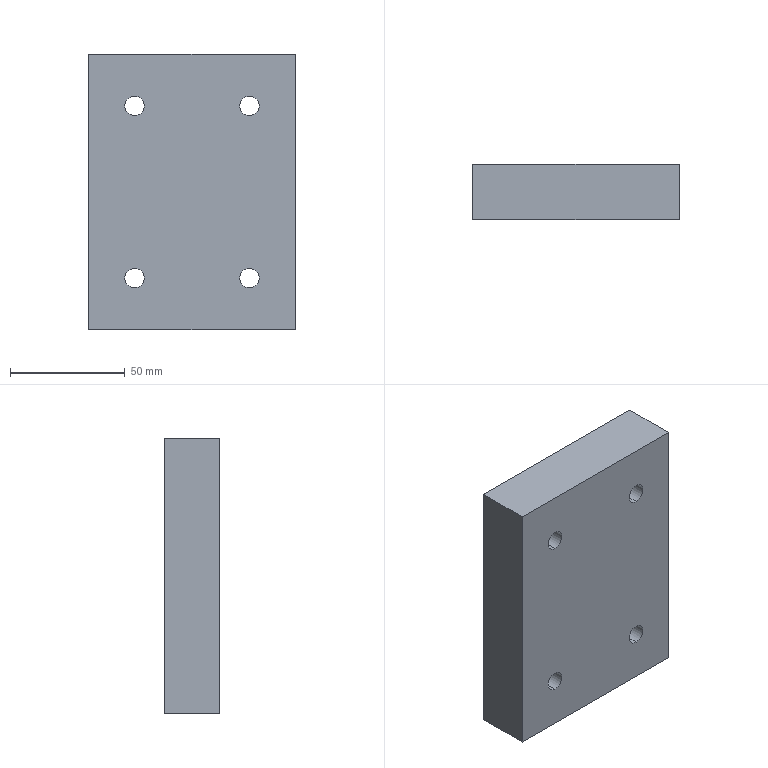Part | SolidWorks | features Extrusion 1, HoleWzd 1 | 1 solid | 14 faces | box 90 x 24 x 120 mm | volume 253752 mm3 | cylinder 8 | plane 6 | commonest cylinder face diameters 8.5 x8
STEP:
#1=CARTESIAN_POINT('',(-25.,0.,33.25));
#2=VERTEX_POINT('',#1);
#3=CARTESIAN_POINT('',(-25.,0.,41.75));
#4=VERTEX_POINT('',#3);
#5=CARTESIAN_POINT('',(-25.,0.,37.5));
#6=DIRECTION('',(0.,1.,0.));
#7=DIRECTION('',(0.,0.,1.));
#8=AXIS2_PLACEMENT_3D('',#5,#6,#7);
#9=CIRCLE('',#8,4.25);
#10=EDGE_CURVE('',#2,#4,#9,.T.);
#11=ORIENTED_EDGE('',*,*,#10,.F.);
#12=CARTESIAN_POINT('',(-25.,24.,33.25));
#13=VERTEX_POINT('',#12);
#14=CARTESIAN_POINT('',(-25.,24.,33.25));
#15=DIRECTION('',(0.,1.,0.));
#16=VECTOR('',#15,1000.);
#17=LINE('',#14,#16);
#18=EDGE_CURVE('',#2,#13,#17,.T.);
#19=ORIENTED_EDGE('',*,*,#18,.T.);
#20=CARTESIAN_POINT('',(-25.,24.,41.75));
#21=VERTEX_POINT('',#20);
#22=CARTESIAN_POINT('',(-25.,24.,37.5));
#23=DIRECTION('',(0.,1.,0.));
#24=DIRECTION('',(0.,0.,1.));
#25=AXIS2_PLACEMENT_3D('',#22,#23,#24);
#26=CIRCLE('',#25,4.25);
#27=EDGE_CURVE('',#13,#21,#26,.T.);
#28=ORIENTED_EDGE('',*,*,#27,.T.);
#29=CARTESIAN_POINT('',(-25.,24.,41.75));
#30=DIRECTION('',(0.,1.,0.));
#31=VECTOR('',#30,1000.);
#32=LINE('',#29,#31);
#33=EDGE_CURVE('',#4,#21,#32,.T.);
#34=ORIENTED_EDGE('',*,*,#33,.F.);
#35=EDGE_LOOP('',(#11,#19,#28,#34));
#36=FACE_OUTER_BOUND('',#35,.T.);
#37=CARTESIAN_POINT('',(-25.,24.,37.5));
#38=DIRECTION('',(0.,1.,0.));
#39=DIRECTION('',(0.,0.,1.));
#40=AXIS2_PLACEMENT_3D('',#37,#38,#39);
#41=CYLINDRICAL_SURFACE('',#40,4.25);
#42=ADVANCED_FACE('',(#36),#41,.F.);
#43=CARTESIAN_POINT('',(-25.,0.,-41.75));
#44=VERTEX_POINT('',#43);
#45=CARTESIAN_POINT('',(-25.,0.,-33.25));
#46=VERTEX_POINT('',#45);
#47=CARTESIAN_POINT('',(-25.,0.,-37.5));
#48=DIRECTION('',(0.,1.,0.));
#49=DIRECTION('',(0.,0.,1.));
#50=AXIS2_PLACEMENT_3D('',#47,#48,#49);
#51=CIRCLE('',#50,4.25);
#52=EDGE_CURVE('',#44,#46,#51,.T.);
#53=ORIENTED_EDGE('',*,*,#52,.F.);
#54=CARTESIAN_POINT('',(-25.,24.,-41.75));
#55=VERTEX_POINT('',#54);
#56=CARTESIAN_POINT('',(-25.,24.,-41.75));
#57=DIRECTION('',(0.,1.,0.));
#58=VECTOR('',#57,1000.);
#59=LINE('',#56,#58);
#60=EDGE_CURVE('',#44,#55,#59,.T.);
#61=ORIENTED_EDGE('',*,*,#60,.T.);
#62=CARTESIAN_POINT('',(-25.,24.,-33.25));
#63=VERTEX_POINT('',#62);
#64=CARTESIAN_POINT('',(-25.,24.,-37.5));
#65=DIRECTION('',(0.,1.,0.));
#66=DIRECTION('',(0.,0.,1.));
#67=AXIS2_PLACEMENT_3D('',#64,#65,#66);
#68=CIRCLE('',#67,4.25);
#69=EDGE_CURVE('',#55,#63,#68,.T.);
#70=ORIENTED_EDGE('',*,*,#69,.T.);
#71=CARTESIAN_POINT('',(-25.,24.,-33.25));
#72=DIRECTION('',(0.,1.,0.));
#73=VECTOR('',#72,1000.);
#74=LINE('',#71,#73);
#75=EDGE_CURVE('',#46,#63,#74,.T.);
#76=ORIENTED_EDGE('',*,*,#75,.F.);
#77=EDGE_LOOP('',(#53,#61,#70,#76));
#78=FACE_OUTER_BOUND('',#77,.T.);
#79=CARTESIAN_POINT('',(-25.,24.,-37.5));
#80=DIRECTION('',(0.,1.,0.));
#81=DIRECTION('',(0.,0.,1.));
#82=AXIS2_PLACEMENT_3D('',#79,#80,#81);
#83=CYLINDRICAL_SURFACE('',#82,4.25);
#84=ADVANCED_FACE('',(#78),#83,.F.);
#85=CARTESIAN_POINT('',(25.,0.,-41.75));
#86=VERTEX_POINT('',#85);
#87=CARTESIAN_POINT('',(25.,0.,-33.25));
#88=VERTEX_POINT('',#87);
#89=CARTESIAN_POINT('',(25.,0.,-37.5));
#90=DIRECTION('',(0.,1.,0.));
#91=DIRECTION('',(0.,0.,1.));
#92=AXIS2_PLACEMENT_3D('',#89,#90,#91);
#93=CIRCLE('',#92,4.25);
#94=EDGE_CURVE('',#86,#88,#93,.T.);
#95=ORIENTED_EDGE('',*,*,#94,.F.);
#96=CARTESIAN_POINT('',(25.,24.,-41.75));
#97=VERTEX_POINT('',#96);
#98=CARTESIAN_POINT('',(25.,24.,-41.75));
#99=DIRECTION('',(0.,1.,0.));
#100=VECTOR('',#99,1000.);
#101=LINE('',#98,#100);
#102=EDGE_CURVE('',#86,#97,#101,.T.);
#103=ORIENTED_EDGE('',*,*,#102,.T.);
#104=CARTESIAN_POINT('',(25.,24.,-33.25));
#105=VERTEX_POINT('',#104);
#106=CARTESIAN_POINT('',(25.,24.,-37.5));
#107=DIRECTION('',(0.,1.,0.));
#108=DIRECTION('',(0.,0.,1.));
#109=AXIS2_PLACEMENT_3D('',#106,#107,#108);
#110=CIRCLE('',#109,4.25);
#111=EDGE_CURVE('',#97,#105,#110,.T.);
#112=ORIENTED_EDGE('',*,*,#111,.T.);
#113=CARTESIAN_POINT('',(25.,24.,-33.25));
#114=DIRECTION('',(0.,1.,0.));
#115=VECTOR('',#114,1000.);
#116=LINE('',#113,#115);
#117=EDGE_CURVE('',#88,#105,#116,.T.);
#118=ORIENTED_EDGE('',*,*,#117,.F.);
#119=EDGE_LOOP('',(#95,#103,#112,#118));
#120=FACE_OUTER_BOUND('',#119,.T.);
#121=CARTESIAN_POINT('',(25.,24.,-37.5));
#122=DIRECTION('',(0.,1.,0.));
#123=DIRECTION('',(0.,0.,1.));
#124=AXIS2_PLACEMENT_3D('',#121,#122,#123);
#125=CYLINDRICAL_SURFACE('',#124,4.25);
#126=ADVANCED_FACE('',(#120),#125,.F.);
#127=CARTESIAN_POINT('',(25.,0.,33.25));
#128=VERTEX_POINT('',#127);
#129=CARTESIAN_POINT('',(25.,0.,41.75));
#130=VERTEX_POINT('',#129);
#131=CARTESIAN_POINT('',(25.,0.,37.5));
#132=DIRECTION('',(0.,1.,0.));
#133=DIRECTION('',(0.,0.,1.));
#134=AXIS2_PLACEMENT_3D('',#131,#132,#133);
#135=CIRCLE('',#134,4.25);
#136=EDGE_CURVE('',#128,#130,#135,.T.);
#137=ORIENTED_EDGE('',*,*,#136,.F.);
#138=CARTESIAN_POINT('',(25.,24.,33.25));
#139=VERTEX_POINT('',#138);
#140=CARTESIAN_POINT('',(25.,24.,33.25));
#141=DIRECTION('',(0.,1.,0.));
#142=VECTOR('',#141,1000.);
#143=LINE('',#140,#142);
#144=EDGE_CURVE('',#128,#139,#143,.T.);
#145=ORIENTED_EDGE('',*,*,#144,.T.);
#146=CARTESIAN_POINT('',(25.,24.,41.75));
#147=VERTEX_POINT('',#146);
#148=CARTESIAN_POINT('',(25.,24.,37.5));
#149=DIRECTION('',(0.,1.,0.));
#150=DIRECTION('',(0.,0.,1.));
#151=AXIS2_PLACEMENT_3D('',#148,#149,#150);
#152=CIRCLE('',#151,4.25);
#153=EDGE_CURVE('',#139,#147,#152,.T.);
#154=ORIENTED_EDGE('',*,*,#153,.T.);
#155=CARTESIAN_POINT('',(25.,24.,41.75));
#156=DIRECTION('',(0.,1.,0.));
#157=VECTOR('',#156,1000.);
#158=LINE('',#155,#157);
#159=EDGE_CURVE('',#130,#147,#158,.T.);
#160=ORIENTED_EDGE('',*,*,#159,.F.);
#161=EDGE_LOOP('',(#137,#145,#154,#160));
#162=FACE_OUTER_BOUND('',#161,.T.);
#163=CARTESIAN_POINT('',(25.,24.,37.5));
#164=DIRECTION('',(0.,1.,0.));
#165=DIRECTION('',(0.,0.,1.));
#166=AXIS2_PLACEMENT_3D('',#163,#164,#165);
#167=CYLINDRICAL_SURFACE('',#166,4.25);
#168=ADVANCED_FACE('',(#162),#167,.F.);
#169=CARTESIAN_POINT('',(45.,0.,60.));
#170=VERTEX_POINT('',#169);
#171=CARTESIAN_POINT('',(45.,0.,-60.));
#172=VERTEX_POINT('',#171);
#173=CARTESIAN_POINT('',(45.,0.,60.));
#174=DIRECTION('',(0.,0.,-1.));
#175=VECTOR('',#174,1000.);
#176=LINE('',#173,#175);
#177=EDGE_CURVE('',#170,#172,#176,.T.);
#178=ORIENTED_EDGE('',*,*,#177,.T.);
#179=CARTESIAN_POINT('',(45.,24.,-60.));
#180=VERTEX_POINT('',#179);
#181=CARTESIAN_POINT('',(45.,24.,-60.));
#182=DIRECTION('',(0.,-1.,0.));
#183=VECTOR('',#182,1000.);
#184=LINE('',#181,#183);
#185=EDGE_CURVE('',#180,#172,#184,.T.);
#186=ORIENTED_EDGE('',*,*,#185,.F.);
#187=CARTESIAN_POINT('',(45.,24.,60.));
#188=VERTEX_POINT('',#187);
#189=CARTESIAN_POINT('',(45.,24.,60.));
#190=DIRECTION('',(0.,0.,-1.));
#191=VECTOR('',#190,1000.);
#192=LINE('',#189,#191);
#193=EDGE_CURVE('',#188,#180,#192,.T.);
#194=ORIENTED_EDGE('',*,*,#193,.F.);
#195=CARTESIAN_POINT('',(45.,24.,60.));
#196=DIRECTION('',(0.,-1.,0.));
#197=VECTOR('',#196,1000.);
#198=LINE('',#195,#197);
#199=EDGE_CURVE('',#188,#170,#198,.T.);
#200=ORIENTED_EDGE('',*,*,#199,.T.);
#201=EDGE_LOOP('',(#178,#186,#194,#200));
#202=FACE_OUTER_BOUND('',#201,.T.);
#203=CARTESIAN_POINT('',(45.,24.,60.));
#204=DIRECTION('',(-1.,0.,0.));
#205=DIRECTION('',(0.,0.,1.));
#206=AXIS2_PLACEMENT_3D('',#203,#204,#205);
#207=PLANE('',#206);
#208=ADVANCED_FACE('',(#202),#207,.F.);
#209=CARTESIAN_POINT('',(-45.,0.,-60.));
#210=VERTEX_POINT('',#209);
#211=CARTESIAN_POINT('',(-45.,0.,-60.));
#212=DIRECTION('',(-1.,0.,0.));
#213=VECTOR('',#212,1000.);
#214=LINE('',#211,#213);
#215=EDGE_CURVE('',#172,#210,#214,.T.);
#216=ORIENTED_EDGE('',*,*,#215,.T.);
#217=CARTESIAN_POINT('',(-45.,24.,-60.));
#218=VERTEX_POINT('',#217);
#219=CARTESIAN_POINT('',(-45.,24.,-60.));
#220=DIRECTION('',(0.,-1.,0.));
#221=VECTOR('',#220,1000.);
#222=LINE('',#219,#221);
#223=EDGE_CURVE('',#218,#210,#222,.T.);
#224=ORIENTED_EDGE('',*,*,#223,.F.);
#225=CARTESIAN_POINT('',(-45.,24.,-60.));
#226=DIRECTION('',(-1.,0.,0.));
#227=VECTOR('',#226,1000.);
#228=LINE('',#225,#227);
#229=EDGE_CURVE('',#180,#218,#228,.T.);
#230=ORIENTED_EDGE('',*,*,#229,.F.);
#231=ORIENTED_EDGE('',*,*,#185,.T.);
#232=EDGE_LOOP('',(#216,#224,#230,#231));
#233=FACE_OUTER_BOUND('',#232,.T.);
#234=CARTESIAN_POINT('',(-45.,24.,-60.));
#235=DIRECTION('',(0.,0.,1.));
#236=DIRECTION('',(1.,0.,0.));
#237=AXIS2_PLACEMENT_3D('',#234,#235,#236);
#238=PLANE('',#237);
#239=ADVANCED_FACE('',(#233),#238,.F.);
#240=CARTESIAN_POINT('',(-45.,0.,60.));
#241=VERTEX_POINT('',#240);
#242=CARTESIAN_POINT('',(-45.,0.,60.));
#243=DIRECTION('',(0.,0.,1.));
#244=VECTOR('',#243,1000.);
#245=LINE('',#242,#244);
#246=EDGE_CURVE('',#210,#241,#245,.T.);
#247=ORIENTED_EDGE('',*,*,#246,.T.);
#248=CARTESIAN_POINT('',(-45.,24.,60.));
#249=VERTEX_POINT('',#248);
#250=CARTESIAN_POINT('',(-45.,24.,60.));
#251=DIRECTION('',(0.,-1.,0.));
#252=VECTOR('',#251,1000.);
#253=LINE('',#250,#252);
#254=EDGE_CURVE('',#249,#241,#253,.T.);
#255=ORIENTED_EDGE('',*,*,#254,.F.);
#256=CARTESIAN_POINT('',(-45.,24.,60.));
#257=DIRECTION('',(0.,0.,1.));
#258=VECTOR('',#257,1000.);
#259=LINE('',#256,#258);
#260=EDGE_CURVE('',#218,#249,#259,.T.);
#261=ORIENTED_EDGE('',*,*,#260,.F.);
#262=ORIENTED_EDGE('',*,*,#223,.T.);
#263=EDGE_LOOP('',(#247,#255,#261,#262));
#264=FACE_OUTER_BOUND('',#263,.T.);
#265=CARTESIAN_POINT('',(-45.,24.,60.));
#266=DIRECTION('',(1.,0.,0.));
#267=DIRECTION('',(0.,0.,-1.));
#268=AXIS2_PLACEMENT_3D('',#265,#266,#267);
#269=PLANE('',#268);
#270=ADVANCED_FACE('',(#264),#269,.F.);
#271=CARTESIAN_POINT('',(-45.,0.,60.));
#272=DIRECTION('',(1.,0.,0.));
#273=VECTOR('',#272,1000.);
#274=LINE('',#271,#273);
#275=EDGE_CURVE('',#241,#170,#274,.T.);
#276=ORIENTED_EDGE('',*,*,#275,.T.);
#277=ORIENTED_EDGE('',*,*,#199,.F.);
#278=CARTESIAN_POINT('',(-45.,24.,60.));
#279=DIRECTION('',(1.,0.,0.));
#280=VECTOR('',#279,1000.);
#281=LINE('',#278,#280);
#282=EDGE_CURVE('',#249,#188,#281,.T.);
#283=ORIENTED_EDGE('',*,*,#282,.F.);
#284=ORIENTED_EDGE('',*,*,#254,.T.);
#285=EDGE_LOOP('',(#276,#277,#283,#284));
#286=FACE_OUTER_BOUND('',#285,.T.);
#287=CARTESIAN_POINT('',(-45.,24.,60.));
#288=DIRECTION('',(0.,0.,-1.));
#289=DIRECTION('',(-1.,0.,0.));
#290=AXIS2_PLACEMENT_3D('',#287,#288,#289);
#291=PLANE('',#290);
#292=ADVANCED_FACE('',(#286),#291,.F.);
#293=CARTESIAN_POINT('',(-25.,24.,37.5));
#294=DIRECTION('',(0.,1.,0.));
#295=DIRECTION('',(0.,0.,1.));
#296=AXIS2_PLACEMENT_3D('',#293,#294,#295);
#297=CIRCLE('',#296,4.25);
#298=EDGE_CURVE('',#21,#13,#297,.T.);
#299=ORIENTED_EDGE('',*,*,#298,.F.);
#300=ORIENTED_EDGE('',*,*,#27,.F.);
#301=EDGE_LOOP('',(#299,#300));
#302=FACE_BOUND('',#301,.T.);
#303=CARTESIAN_POINT('',(-25.,24.,-37.5));
#304=DIRECTION('',(0.,1.,0.));
#305=DIRECTION('',(0.,0.,1.));
#306=AXIS2_PLACEMENT_3D('',#303,#304,#305);
#307=CIRCLE('',#306,4.25);
#308=EDGE_CURVE('',#63,#55,#307,.T.);
#309=ORIENTED_EDGE('',*,*,#308,.F.);
#310=ORIENTED_EDGE('',*,*,#69,.F.);
#311=EDGE_LOOP('',(#309,#310));
#312=FACE_BOUND('',#311,.T.);
#313=CARTESIAN_POINT('',(25.,24.,-37.5));
#314=DIRECTION('',(0.,1.,0.));
#315=DIRECTION('',(0.,0.,1.));
#316=AXIS2_PLACEMENT_3D('',#313,#314,#315);
#317=CIRCLE('',#316,4.25);
#318=EDGE_CURVE('',#105,#97,#317,.T.);
#319=ORIENTED_EDGE('',*,*,#318,.F.);
#320=ORIENTED_EDGE('',*,*,#111,.F.);
#321=EDGE_LOOP('',(#319,#320));
#322=FACE_BOUND('',#321,.T.);
#323=CARTESIAN_POINT('',(25.,24.,37.5));
#324=DIRECTION('',(0.,1.,0.));
#325=DIRECTION('',(0.,0.,1.));
#326=AXIS2_PLACEMENT_3D('',#323,#324,#325);
#327=CIRCLE('',#326,4.25);
#328=EDGE_CURVE('',#147,#139,#327,.T.);
#329=ORIENTED_EDGE('',*,*,#328,.F.);
#330=ORIENTED_EDGE('',*,*,#153,.F.);
#331=EDGE_LOOP('',(#329,#330));
#332=FACE_BOUND('',#331,.T.);
#333=ORIENTED_EDGE('',*,*,#193,.T.);
#334=ORIENTED_EDGE('',*,*,#229,.T.);
#335=ORIENTED_EDGE('',*,*,#260,.T.);
#336=ORIENTED_EDGE('',*,*,#282,.T.);
#337=EDGE_LOOP('',(#333,#334,#335,#336));
#338=FACE_OUTER_BOUND('',#337,.T.);
#339=CARTESIAN_POINT('',(0.,24.,0.));
#340=DIRECTION('',(0.,-1.,0.));
#341=DIRECTION('',(0.,0.,-1.));
#342=AXIS2_PLACEMENT_3D('',#339,#340,#341);
#343=PLANE('',#342);
#344=ADVANCED_FACE('',(#302,#312,#322,#332,#338),#343,.F.);
#345=CARTESIAN_POINT('',(-25.,0.,37.5));
#346=DIRECTION('',(0.,1.,0.));
#347=DIRECTION('',(0.,0.,1.));
#348=AXIS2_PLACEMENT_3D('',#345,#346,#347);
#349=CIRCLE('',#348,4.25);
#350=EDGE_CURVE('',#4,#2,#349,.T.);
#351=ORIENTED_EDGE('',*,*,#350,.T.);
#352=ORIENTED_EDGE('',*,*,#10,.T.);
#353=EDGE_LOOP('',(#351,#352));
#354=FACE_BOUND('',#353,.T.);
#355=CARTESIAN_POINT('',(-25.,0.,-37.5));
#356=DIRECTION('',(0.,1.,0.));
#357=DIRECTION('',(0.,0.,1.));
#358=AXIS2_PLACEMENT_3D('',#355,#356,#357);
#359=CIRCLE('',#358,4.25);
#360=EDGE_CURVE('',#46,#44,#359,.T.);
#361=ORIENTED_EDGE('',*,*,#360,.T.);
#362=ORIENTED_EDGE('',*,*,#52,.T.);
#363=EDGE_LOOP('',(#361,#362));
#364=FACE_BOUND('',#363,.T.);
#365=CARTESIAN_POINT('',(25.,0.,-37.5));
#366=DIRECTION('',(0.,1.,0.));
#367=DIRECTION('',(0.,0.,1.));
#368=AXIS2_PLACEMENT_3D('',#365,#366,#367);
#369=CIRCLE('',#368,4.25);
#370=EDGE_CURVE('',#88,#86,#369,.T.);
#371=ORIENTED_EDGE('',*,*,#370,.T.);
#372=ORIENTED_EDGE('',*,*,#94,.T.);
#373=EDGE_LOOP('',(#371,#372));
#374=FACE_BOUND('',#373,.T.);
#375=CARTESIAN_POINT('',(25.,0.,37.5));
#376=DIRECTION('',(0.,1.,0.));
#377=DIRECTION('',(0.,0.,1.));
#378=AXIS2_PLACEMENT_3D('',#375,#376,#377);
#379=CIRCLE('',#378,4.25);
#380=EDGE_CURVE('',#130,#128,#379,.T.);
#381=ORIENTED_EDGE('',*,*,#380,.T.);
#382=ORIENTED_EDGE('',*,*,#136,.T.);
#383=EDGE_LOOP('',(#381,#382));
#384=FACE_BOUND('',#383,.T.);
#385=ORIENTED_EDGE('',*,*,#177,.F.);
#386=ORIENTED_EDGE('',*,*,#275,.F.);
#387=ORIENTED_EDGE('',*,*,#246,.F.);
#388=ORIENTED_EDGE('',*,*,#215,.F.);
#389=EDGE_LOOP('',(#385,#386,#387,#388));
#390=FACE_OUTER_BOUND('',#389,.T.);
#391=CARTESIAN_POINT('',(0.,0.,0.));
#392=DIRECTION('',(0.,-1.,0.));
#393=DIRECTION('',(0.,0.,-1.));
#394=AXIS2_PLACEMENT_3D('',#391,#392,#393);
#395=PLANE('',#394);
#396=ADVANCED_FACE('',(#354,#364,#374,#384,#390),#395,.T.);
#397=ORIENTED_EDGE('',*,*,#144,.F.);
#398=ORIENTED_EDGE('',*,*,#380,.F.);
#399=ORIENTED_EDGE('',*,*,#159,.T.);
#400=ORIENTED_EDGE('',*,*,#328,.T.);
#401=EDGE_LOOP('',(#397,#398,#399,#400));
#402=FACE_OUTER_BOUND('',#401,.T.);
#403=CARTESIAN_POINT('',(25.,24.,37.5));
#404=DIRECTION('',(0.,1.,0.));
#405=DIRECTION('',(0.,0.,1.));
#406=AXIS2_PLACEMENT_3D('',#403,#404,#405);
#407=CYLINDRICAL_SURFACE('',#406,4.25);
#408=ADVANCED_FACE('',(#402),#407,.F.);
#409=ORIENTED_EDGE('',*,*,#102,.F.);
#410=ORIENTED_EDGE('',*,*,#370,.F.);
#411=ORIENTED_EDGE('',*,*,#117,.T.);
#412=ORIENTED_EDGE('',*,*,#318,.T.);
#413=EDGE_LOOP('',(#409,#410,#411,#412));
#414=FACE_OUTER_BOUND('',#413,.T.);
#415=CARTESIAN_POINT('',(25.,24.,-37.5));
#416=DIRECTION('',(0.,1.,0.));
#417=DIRECTION('',(0.,0.,1.));
#418=AXIS2_PLACEMENT_3D('',#415,#416,#417);
#419=CYLINDRICAL_SURFACE('',#418,4.25);
#420=ADVANCED_FACE('',(#414),#419,.F.);
#421=ORIENTED_EDGE('',*,*,#60,.F.);
#422=ORIENTED_EDGE('',*,*,#360,.F.);
#423=ORIENTED_EDGE('',*,*,#75,.T.);
#424=ORIENTED_EDGE('',*,*,#308,.T.);
#425=EDGE_LOOP('',(#421,#422,#423,#424));
#426=FACE_OUTER_BOUND('',#425,.T.);
#427=CARTESIAN_POINT('',(-25.,24.,-37.5));
#428=DIRECTION('',(0.,1.,0.));
#429=DIRECTION('',(0.,0.,1.));
#430=AXIS2_PLACEMENT_3D('',#427,#428,#429);
#431=CYLINDRICAL_SURFACE('',#430,4.25);
#432=ADVANCED_FACE('',(#426),#431,.F.);
#433=ORIENTED_EDGE('',*,*,#18,.F.);
#434=ORIENTED_EDGE('',*,*,#350,.F.);
#435=ORIENTED_EDGE('',*,*,#33,.T.);
#436=ORIENTED_EDGE('',*,*,#298,.T.);
#437=EDGE_LOOP('',(#433,#434,#435,#436));
#438=FACE_OUTER_BOUND('',#437,.T.);
#439=CARTESIAN_POINT('',(-25.,24.,37.5));
#440=DIRECTION('',(0.,1.,0.));
#441=DIRECTION('',(0.,0.,1.));
#442=AXIS2_PLACEMENT_3D('',#439,#440,#441);
#443=CYLINDRICAL_SURFACE('',#442,4.25);
#444=ADVANCED_FACE('',(#438),#443,.F.);
#445=CLOSED_SHELL('',(#42,#84,#126,#168,#208,#239,#270,#292,#344,#396,#408,#420,#432,#444));
#446=MANIFOLD_SOLID_BREP('',#445);
#447=CARTESIAN_POINT('',(0.,0.,0.));
#448=DIRECTION('',(0.,0.,1.));
#449=DIRECTION('',(1.,0.,0.));
#450=AXIS2_PLACEMENT_3D('',#447,#448,#449);
#451=(LENGTH_UNIT()NAMED_UNIT(*)SI_UNIT(.MILLI.,.METRE.));
#452=UNCERTAINTY_MEASURE_WITH_UNIT(LENGTH_MEASURE(0.00001),#451,'','');
#453=(NAMED_UNIT(*)PLANE_ANGLE_UNIT()SI_UNIT($,.RADIAN.));
#454=(NAMED_UNIT(*)SI_UNIT($,.STERADIAN.)SOLID_ANGLE_UNIT());
#455=(GEOMETRIC_REPRESENTATION_CONTEXT(3)GLOBAL_UNCERTAINTY_ASSIGNED_CONTEXT((#452))GLOBAL_UNIT_ASSIGNED_CONTEXT((#451,#453,#454))REPRESENTATION_CONTEXT('',''));
#456=ADVANCED_BREP_SHAPE_REPRESENTATION('',(#446,#450),#455);